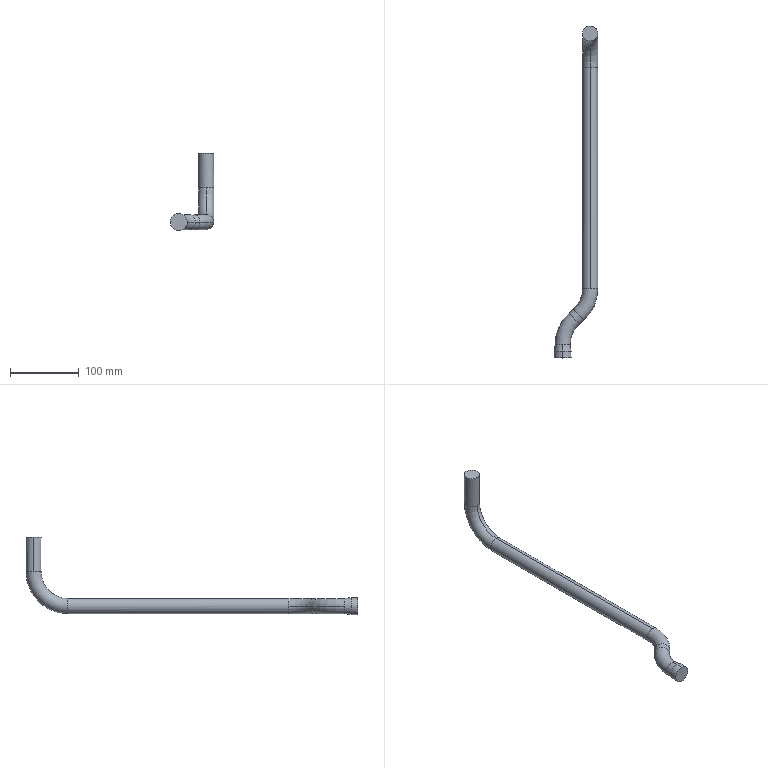Part | STEP file | copper tube 42_default_machined_ | 1 solid | 18 faces | box 63.3 x 483.405 x 112.3 mm | volume 215626 mm3 | cylinder 8 | torus 6 | cone 2 | plane 2 | commonest cylinder face diameters 22 x6 24.6 x2
STEP:
#1=CARTESIAN_POINT('',(0.,0.,0.));
#2=DIRECTION('',(0.,0.,1.));
#3=DIRECTION('',(1.,0.,0.));
#4=AXIS2_PLACEMENT_3D('',#1,#2,#3);
#5=CARTESIAN_POINT('',(380.2,1004.975,11.));
#6=VERTEX_POINT('',#5);
#7=CARTESIAN_POINT('',(380.2,1004.975,-11.));
#8=VERTEX_POINT('',#7);
#9=CARTESIAN_POINT('',(380.2,1004.975,0.));
#10=DIRECTION('',(0.,1.,0.));
#11=DIRECTION('',(-1.,0.,0.));
#12=AXIS2_PLACEMENT_3D('',#9,#10,#11);
#13=CIRCLE('',#12,11.);
#14=CARTESIAN_POINT('',(380.2,1004.975,50.));
#15=DIRECTION('',(1.,0.,0.));
#16=DIRECTION('',(0.,0.,-1.));
#17=AXIS2_PLACEMENT_3D('',#14,#15,#16);
#18=TOROIDAL_SURFACE('',#17,50.,11.);
#19=CARTESIAN_POINT('',(0.,4.712));
#20=DIRECTION('',(0.,-1.));
#21=VECTOR('',#20,1.);
#22=LINE('',#19,#21);
#23=(GEOMETRIC_REPRESENTATION_CONTEXT(2)PARAMETRIC_REPRESENTATION_CONTEXT()REPRESENTATION_CONTEXT('',''));
#24=DEFINITIONAL_REPRESENTATION('',(#22),#23);
#25=PCURVE('',#18,#24);
#26=CARTESIAN_POINT('',(380.2,683.041,0.));
#27=DIRECTION('',(0.,1.,0.));
#28=DIRECTION('',(0.,0.,1.));
#29=AXIS2_PLACEMENT_3D('',#26,#27,#28);
#30=CYLINDRICAL_SURFACE('',#29,11.);
#31=CARTESIAN_POINT('',(-1.571,321.934));
#32=DIRECTION('',(1.,0.));
#33=VECTOR('',#32,1.);
#34=LINE('',#31,#33);
#35=(GEOMETRIC_REPRESENTATION_CONTEXT(2)PARAMETRIC_REPRESENTATION_CONTEXT()REPRESENTATION_CONTEXT('',''));
#36=DEFINITIONAL_REPRESENTATION('',(#34),#35);
#37=PCURVE('',#30,#36);
#38=SURFACE_CURVE('',#13,(#25,#37),.PCURVE_S1.);
#39=EDGE_CURVE('',#6,#8,#38,.T.);
#40=ORIENTED_EDGE('',*,*,#39,.T.);
#41=CARTESIAN_POINT('',(380.2,1065.975,50.));
#42=VERTEX_POINT('',#41);
#43=CARTESIAN_POINT('',(380.2,1004.975,50.));
#44=DIRECTION('',(1.,0.,0.));
#45=DIRECTION('',(0.,0.,-1.));
#46=AXIS2_PLACEMENT_3D('',#43,#44,#45);
#47=CIRCLE('',#46,61.);
#48=CARTESIAN_POINT('',(0.,0.));
#49=DIRECTION('',(1.,0.));
#50=VECTOR('',#49,1.);
#51=LINE('',#48,#50);
#52=(GEOMETRIC_REPRESENTATION_CONTEXT(2)PARAMETRIC_REPRESENTATION_CONTEXT()REPRESENTATION_CONTEXT('',''));
#53=DEFINITIONAL_REPRESENTATION('',(#51),#52);
#54=PCURVE('',#18,#53);
#55=CARTESIAN_POINT('',(380.2,1004.975,50.));
#56=DIRECTION('',(1.,0.,0.));
#57=DIRECTION('',(0.,0.,-1.));
#58=AXIS2_PLACEMENT_3D('',#55,#56,#57);
#59=TOROIDAL_SURFACE('',#58,50.,11.);
#60=CARTESIAN_POINT('',(0.,6.283));
#61=DIRECTION('',(1.,0.));
#62=VECTOR('',#61,1.);
#63=LINE('',#60,#62);
#64=(GEOMETRIC_REPRESENTATION_CONTEXT(2)PARAMETRIC_REPRESENTATION_CONTEXT()REPRESENTATION_CONTEXT('',''));
#65=DEFINITIONAL_REPRESENTATION('',(#63),#64);
#66=PCURVE('',#59,#65);
#67=SURFACE_CURVE('',#47,(#54,#66),.PCURVE_S1.);
#68=EDGE_CURVE('',#8,#42,#67,.T.);
#69=ORIENTED_EDGE('',*,*,#68,.T.);
#70=CARTESIAN_POINT('',(391.2,1054.975,50.));
#71=VERTEX_POINT('',#70);
#72=CARTESIAN_POINT('',(380.2,1054.975,50.));
#73=DIRECTION('',(0.,0.,1.));
#74=DIRECTION('',(-1.,0.,0.));
#75=AXIS2_PLACEMENT_3D('',#72,#73,#74);
#76=CIRCLE('',#75,11.);
#77=CARTESIAN_POINT('',(1.571,4.712));
#78=DIRECTION('',(0.,-1.));
#79=VECTOR('',#78,1.);
#80=LINE('',#77,#79);
#81=(GEOMETRIC_REPRESENTATION_CONTEXT(2)PARAMETRIC_REPRESENTATION_CONTEXT()REPRESENTATION_CONTEXT('',''));
#82=DEFINITIONAL_REPRESENTATION('',(#80),#81);
#83=PCURVE('',#18,#82);
#84=CARTESIAN_POINT('',(380.2,1054.975,50.));
#85=DIRECTION('',(0.,0.,1.));
#86=DIRECTION('',(1.,0.,0.));
#87=AXIS2_PLACEMENT_3D('',#84,#85,#86);
#88=CYLINDRICAL_SURFACE('',#87,11.);
#89=CARTESIAN_POINT('',(-3.142,0.));
#90=DIRECTION('',(1.,0.));
#91=VECTOR('',#90,1.);
#92=LINE('',#89,#91);
#93=(GEOMETRIC_REPRESENTATION_CONTEXT(2)PARAMETRIC_REPRESENTATION_CONTEXT()REPRESENTATION_CONTEXT('',''));
#94=DEFINITIONAL_REPRESENTATION('',(#92),#93);
#95=PCURVE('',#88,#94);
#96=SURFACE_CURVE('',#76,(#83,#95),.PCURVE_S1.);
#97=EDGE_CURVE('',#71,#42,#96,.T.);
#98=ORIENTED_EDGE('',*,*,#97,.F.);
#99=CARTESIAN_POINT('',(380.2,1043.975,50.));
#100=VERTEX_POINT('',#99);
#101=CARTESIAN_POINT('',(380.2,1054.975,50.));
#102=DIRECTION('',(0.,0.,1.));
#103=DIRECTION('',(-1.,0.,0.));
#104=AXIS2_PLACEMENT_3D('',#101,#102,#103);
#105=CIRCLE('',#104,11.);
#106=CARTESIAN_POINT('',(1.571,4.712));
#107=DIRECTION('',(0.,-1.));
#108=VECTOR('',#107,1.);
#109=LINE('',#106,#108);
#110=(GEOMETRIC_REPRESENTATION_CONTEXT(2)PARAMETRIC_REPRESENTATION_CONTEXT()REPRESENTATION_CONTEXT('',''));
#111=DEFINITIONAL_REPRESENTATION('',(#109),#110);
#112=PCURVE('',#18,#111);
#113=CARTESIAN_POINT('',(380.2,1054.975,50.));
#114=DIRECTION('',(0.,0.,1.));
#115=DIRECTION('',(1.,0.,0.));
#116=AXIS2_PLACEMENT_3D('',#113,#114,#115);
#117=CYLINDRICAL_SURFACE('',#116,11.);
#118=CARTESIAN_POINT('',(3.142,0.));
#119=DIRECTION('',(1.,0.));
#120=VECTOR('',#119,1.);
#121=LINE('',#118,#120);
#122=(GEOMETRIC_REPRESENTATION_CONTEXT(2)PARAMETRIC_REPRESENTATION_CONTEXT()REPRESENTATION_CONTEXT('',''));
#123=DEFINITIONAL_REPRESENTATION('',(#121),#122);
#124=PCURVE('',#117,#123);
#125=SURFACE_CURVE('',#105,(#112,#124),.PCURVE_S1.);
#126=EDGE_CURVE('',#100,#71,#125,.T.);
#127=ORIENTED_EDGE('',*,*,#126,.F.);
#128=CARTESIAN_POINT('',(380.2,1004.975,50.));
#129=DIRECTION('',(1.,0.,0.));
#130=DIRECTION('',(0.,0.,-1.));
#131=AXIS2_PLACEMENT_3D('',#128,#129,#130);
#132=CIRCLE('',#131,39.);
#133=CARTESIAN_POINT('',(0.,3.142));
#134=DIRECTION('',(1.,0.));
#135=VECTOR('',#134,1.);
#136=LINE('',#133,#135);
#137=(GEOMETRIC_REPRESENTATION_CONTEXT(2)PARAMETRIC_REPRESENTATION_CONTEXT()REPRESENTATION_CONTEXT('',''));
#138=DEFINITIONAL_REPRESENTATION('',(#136),#137);
#139=PCURVE('',#18,#138);
#140=CARTESIAN_POINT('',(0.,3.142));
#141=DIRECTION('',(1.,0.));
#142=VECTOR('',#141,1.);
#143=LINE('',#140,#142);
#144=(GEOMETRIC_REPRESENTATION_CONTEXT(2)PARAMETRIC_REPRESENTATION_CONTEXT()REPRESENTATION_CONTEXT('',''));
#145=DEFINITIONAL_REPRESENTATION('',(#143),#144);
#146=PCURVE('',#59,#145);
#147=SURFACE_CURVE('',#132,(#139,#146),.PCURVE_S1.);
#148=EDGE_CURVE('',#6,#100,#147,.T.);
#149=ORIENTED_EDGE('',*,*,#148,.F.);
#150=EDGE_LOOP('',(#40,#69,#98,#127,#149));
#151=FACE_BOUND('',#150,.T.);
#152=ADVANCED_FACE('',(#151),#18,.T.);
#153=CARTESIAN_POINT('',(340.2,602.57,-11.));
#154=VERTEX_POINT('',#153);
#155=CARTESIAN_POINT('',(329.2,602.57,0.));
#156=VERTEX_POINT('',#155);
#157=CARTESIAN_POINT('',(340.2,602.57,0.));
#158=DIRECTION('',(0.,1.,0.));
#159=DIRECTION('',(0.,0.,-1.));
#160=AXIS2_PLACEMENT_3D('',#157,#158,#159);
#161=CIRCLE('',#160,11.);
#162=CARTESIAN_POINT('',(390.2,602.57,0.));
#163=DIRECTION('',(0.,0.,-1.));
#164=DIRECTION('',(-1.,0.,0.));
#165=AXIS2_PLACEMENT_3D('',#162,#163,#164);
#166=TOROIDAL_SURFACE('',#165,50.,11.);
#167=CARTESIAN_POINT('',(0.,1.571));
#168=DIRECTION('',(0.,-1.));
#169=VECTOR('',#168,1.);
#170=LINE('',#167,#169);
#171=(GEOMETRIC_REPRESENTATION_CONTEXT(2)PARAMETRIC_REPRESENTATION_CONTEXT()REPRESENTATION_CONTEXT('',''));
#172=DEFINITIONAL_REPRESENTATION('',(#170),#171);
#173=PCURVE('',#166,#172);
#174=CARTESIAN_POINT('',(340.2,592.57,0.));
#175=DIRECTION('',(0.,-1.,0.));
#176=DIRECTION('',(0.,0.,-1.));
#177=AXIS2_PLACEMENT_3D('',#174,#175,#176);
#178=CONICAL_SURFACE('',#177,12.3,0.1293);
#179=CARTESIAN_POINT('',(6.283,-10.));
#180=DIRECTION('',(-1.,0.));
#181=VECTOR('',#180,1.);
#182=LINE('',#179,#181);
#183=(GEOMETRIC_REPRESENTATION_CONTEXT(2)PARAMETRIC_REPRESENTATION_CONTEXT()REPRESENTATION_CONTEXT('',''));
#184=DEFINITIONAL_REPRESENTATION('',(#182),#183);
#185=PCURVE('',#178,#184);
#186=SURFACE_CURVE('',#161,(#173,#185),.PCURVE_S1.);
#187=EDGE_CURVE('',#154,#156,#186,.T.);
#188=ORIENTED_EDGE('',*,*,#187,.T.);
#189=CARTESIAN_POINT('',(349.639,648.131,0.));
#190=VERTEX_POINT('',#189);
#191=CARTESIAN_POINT('',(390.2,602.57,0.));
#192=DIRECTION('',(0.,0.,-1.));
#193=DIRECTION('',(-1.,0.,0.));
#194=AXIS2_PLACEMENT_3D('',#191,#192,#193);
#195=CIRCLE('',#194,61.);
#196=CARTESIAN_POINT('',(0.,0.));
#197=DIRECTION('',(1.,0.));
#198=VECTOR('',#197,1.);
#199=LINE('',#196,#198);
#200=(GEOMETRIC_REPRESENTATION_CONTEXT(2)PARAMETRIC_REPRESENTATION_CONTEXT()REPRESENTATION_CONTEXT('',''));
#201=DEFINITIONAL_REPRESENTATION('',(#199),#200);
#202=PCURVE('',#166,#201);
#203=CARTESIAN_POINT('',(390.2,602.57,0.));
#204=DIRECTION('',(0.,0.,-1.));
#205=DIRECTION('',(-1.,0.,0.));
#206=AXIS2_PLACEMENT_3D('',#203,#204,#205);
#207=TOROIDAL_SURFACE('',#206,50.,11.);
#208=CARTESIAN_POINT('',(0.,6.283));
#209=DIRECTION('',(1.,0.));
#210=VECTOR('',#209,1.);
#211=LINE('',#208,#210);
#212=(GEOMETRIC_REPRESENTATION_CONTEXT(2)PARAMETRIC_REPRESENTATION_CONTEXT()REPRESENTATION_CONTEXT('',''));
#213=DEFINITIONAL_REPRESENTATION('',(#211),#212);
#214=PCURVE('',#207,#213);
#215=SURFACE_CURVE('',#195,(#202,#214),.PCURVE_S1.);
#216=EDGE_CURVE('',#156,#190,#215,.T.);
#217=ORIENTED_EDGE('',*,*,#216,.T.);
#218=CARTESIAN_POINT('',(364.268,631.699,0.));
#219=VERTEX_POINT('',#218);
#220=CARTESIAN_POINT('',(356.953,639.915,0.));
#221=DIRECTION('',(0.7469,0.6649,0.));
#222=DIRECTION('',(-0.6649,0.7469,0.));
#223=AXIS2_PLACEMENT_3D('',#220,#221,#222);
#224=CIRCLE('',#223,11.);
#225=CARTESIAN_POINT('',(0.8434,6.283));
#226=DIRECTION('',(0.,-1.));
#227=VECTOR('',#226,1.);
#228=LINE('',#225,#227);
#229=(GEOMETRIC_REPRESENTATION_CONTEXT(2)PARAMETRIC_REPRESENTATION_CONTEXT()REPRESENTATION_CONTEXT('',''));
#230=DEFINITIONAL_REPRESENTATION('',(#228),#229);
#231=PCURVE('',#166,#230);
#232=CARTESIAN_POINT('',(356.953,639.915,0.));
#233=DIRECTION('',(0.7469,0.6649,0.));
#234=DIRECTION('',(-0.6649,0.7469,0.));
#235=AXIS2_PLACEMENT_3D('',#232,#233,#234);
#236=CYLINDRICAL_SURFACE('',#235,11.);
#237=CARTESIAN_POINT('',(0.,0.));
#238=DIRECTION('',(1.,0.));
#239=VECTOR('',#238,1.);
#240=LINE('',#237,#239);
#241=(GEOMETRIC_REPRESENTATION_CONTEXT(2)PARAMETRIC_REPRESENTATION_CONTEXT()REPRESENTATION_CONTEXT('',''));
#242=DEFINITIONAL_REPRESENTATION('',(#240),#241);
#243=PCURVE('',#236,#242);
#244=SURFACE_CURVE('',#224,(#231,#243),.PCURVE_S1.);
#245=EDGE_CURVE('',#219,#190,#244,.T.);
#246=ORIENTED_EDGE('',*,*,#245,.F.);
#247=CARTESIAN_POINT('',(351.2,602.57,0.));
#248=VERTEX_POINT('',#247);
#249=CARTESIAN_POINT('',(390.2,602.57,0.));
#250=DIRECTION('',(0.,0.,-1.));
#251=DIRECTION('',(-1.,0.,0.));
#252=AXIS2_PLACEMENT_3D('',#249,#250,#251);
#253=CIRCLE('',#252,39.);
#254=CARTESIAN_POINT('',(0.,3.142));
#255=DIRECTION('',(1.,0.));
#256=VECTOR('',#255,1.);
#257=LINE('',#254,#256);
#258=(GEOMETRIC_REPRESENTATION_CONTEXT(2)PARAMETRIC_REPRESENTATION_CONTEXT()REPRESENTATION_CONTEXT('',''));
#259=DEFINITIONAL_REPRESENTATION('',(#257),#258);
#260=PCURVE('',#166,#259);
#261=CARTESIAN_POINT('',(0.,3.142));
#262=DIRECTION('',(1.,0.));
#263=VECTOR('',#262,1.);
#264=LINE('',#261,#263);
#265=(GEOMETRIC_REPRESENTATION_CONTEXT(2)PARAMETRIC_REPRESENTATION_CONTEXT()REPRESENTATION_CONTEXT('',''));
#266=DEFINITIONAL_REPRESENTATION('',(#264),#265);
#267=PCURVE('',#207,#266);
#268=SURFACE_CURVE('',#253,(#260,#267),.PCURVE_S1.);
#269=EDGE_CURVE('',#248,#219,#268,.T.);
#270=ORIENTED_EDGE('',*,*,#269,.F.);
#271=CARTESIAN_POINT('',(340.2,602.57,0.));
#272=DIRECTION('',(0.,1.,0.));
#273=DIRECTION('',(0.,0.,-1.));
#274=AXIS2_PLACEMENT_3D('',#271,#272,#273);
#275=CIRCLE('',#274,11.);
#276=CARTESIAN_POINT('',(0.,7.854));
#277=DIRECTION('',(0.,-1.));
#278=VECTOR('',#277,1.);
#279=LINE('',#276,#278);
#280=(GEOMETRIC_REPRESENTATION_CONTEXT(2)PARAMETRIC_REPRESENTATION_CONTEXT()REPRESENTATION_CONTEXT('',''));
#281=DEFINITIONAL_REPRESENTATION('',(#279),#280);
#282=PCURVE('',#166,#281);
#283=CARTESIAN_POINT('',(340.2,592.57,0.));
#284=DIRECTION('',(0.,-1.,0.));
#285=DIRECTION('',(0.,0.,-1.));
#286=AXIS2_PLACEMENT_3D('',#283,#284,#285);
#287=CONICAL_SURFACE('',#286,12.3,0.1293);
#288=CARTESIAN_POINT('',(6.283,-10.));
#289=DIRECTION('',(-1.,0.));
#290=VECTOR('',#289,1.);
#291=LINE('',#288,#290);
#292=(GEOMETRIC_REPRESENTATION_CONTEXT(2)PARAMETRIC_REPRESENTATION_CONTEXT()REPRESENTATION_CONTEXT('',''));
#293=DEFINITIONAL_REPRESENTATION('',(#291),#292);
#294=PCURVE('',#287,#293);
#295=SURFACE_CURVE('',#275,(#282,#294),.PCURVE_S1.);
#296=EDGE_CURVE('',#248,#154,#295,.T.);
#297=ORIENTED_EDGE('',*,*,#296,.T.);
#298=EDGE_LOOP('',(#188,#217,#246,#270,#297));
#299=FACE_BOUND('',#298,.T.);
#300=ADVANCED_FACE('',(#299),#166,.T.);
#301=CARTESIAN_POINT('',(356.132,653.912,0.));
#302=VERTEX_POINT('',#301);
#303=CARTESIAN_POINT('',(370.761,637.48,0.));
#304=VERTEX_POINT('',#303);
#305=CARTESIAN_POINT('',(363.447,645.696,0.));
#306=DIRECTION('',(0.7469,0.6649,0.));
#307=DIRECTION('',(-0.6649,0.7469,0.));
#308=AXIS2_PLACEMENT_3D('',#305,#306,#307);
#309=CIRCLE('',#308,11.);
#310=CARTESIAN_POINT('',(330.2,683.041,0.));
#311=DIRECTION('',(0.,0.,1.));
#312=DIRECTION('',(1.,0.,0.));
#313=AXIS2_PLACEMENT_3D('',#310,#311,#312);
#314=TOROIDAL_SURFACE('',#313,50.,11.);
#315=CARTESIAN_POINT('',(5.44,3.142));
#316=DIRECTION('',(0.,-1.));
#317=VECTOR('',#316,1.);
#318=LINE('',#315,#317);
#319=(GEOMETRIC_REPRESENTATION_CONTEXT(2)PARAMETRIC_REPRESENTATION_CONTEXT()REPRESENTATION_CONTEXT('',''));
#320=DEFINITIONAL_REPRESENTATION('',(#318),#319);
#321=PCURVE('',#314,#320);
#322=CARTESIAN_POINT('',(356.953,639.915,0.));
#323=DIRECTION('',(0.7469,0.6649,0.));
#324=DIRECTION('',(-0.6649,0.7469,0.));
#325=AXIS2_PLACEMENT_3D('',#322,#323,#324);
#326=CYLINDRICAL_SURFACE('',#325,11.);
#327=CARTESIAN_POINT('',(0.,8.694));
#328=DIRECTION('',(1.,0.));
#329=VECTOR('',#328,1.);
#330=LINE('',#327,#329);
#331=(GEOMETRIC_REPRESENTATION_CONTEXT(2)PARAMETRIC_REPRESENTATION_CONTEXT()REPRESENTATION_CONTEXT('',''));
#332=DEFINITIONAL_REPRESENTATION('',(#330),#331);
#333=PCURVE('',#326,#332);
#334=SURFACE_CURVE('',#309,(#321,#333),.PCURVE_S1.);
#335=EDGE_CURVE('',#302,#304,#334,.T.);
#336=ORIENTED_EDGE('',*,*,#335,.T.);
#337=CARTESIAN_POINT('',(391.2,683.041,0.));
#338=VERTEX_POINT('',#337);
#339=CARTESIAN_POINT('',(330.2,683.041,0.));
#340=DIRECTION('',(0.,0.,1.));
#341=DIRECTION('',(1.,0.,0.));
#342=AXIS2_PLACEMENT_3D('',#339,#340,#341);
#343=CIRCLE('',#342,61.);
#344=CARTESIAN_POINT('',(0.,0.));
#345=DIRECTION('',(1.,0.));
#346=VECTOR('',#345,1.);
#347=LINE('',#344,#346);
#348=(GEOMETRIC_REPRESENTATION_CONTEXT(2)PARAMETRIC_REPRESENTATION_CONTEXT()REPRESENTATION_CONTEXT('',''));
#349=DEFINITIONAL_REPRESENTATION('',(#347),#348);
#350=PCURVE('',#314,#349);
#351=CARTESIAN_POINT('',(330.2,683.041,0.));
#352=DIRECTION('',(0.,0.,1.));
#353=DIRECTION('',(1.,0.,0.));
#354=AXIS2_PLACEMENT_3D('',#351,#352,#353);
#355=TOROIDAL_SURFACE('',#354,50.,11.);
#356=CARTESIAN_POINT('',(0.,6.283));
#357=DIRECTION('',(1.,0.));
#358=VECTOR('',#357,1.);
#359=LINE('',#356,#358);
#360=(GEOMETRIC_REPRESENTATION_CONTEXT(2)PARAMETRIC_REPRESENTATION_CONTEXT()REPRESENTATION_CONTEXT('',''));
#361=DEFINITIONAL_REPRESENTATION('',(#359),#360);
#362=PCURVE('',#355,#361);
#363=SURFACE_CURVE('',#343,(#350,#362),.PCURVE_S1.);
#364=EDGE_CURVE('',#304,#338,#363,.T.);
#365=ORIENTED_EDGE('',*,*,#364,.T.);
#366=CARTESIAN_POINT('',(380.2,683.041,11.));
#367=VERTEX_POINT('',#366);
#368=CARTESIAN_POINT('',(380.2,683.041,0.));
#369=DIRECTION('',(0.,1.,0.));
#370=DIRECTION('',(-1.,0.,0.));
#371=AXIS2_PLACEMENT_3D('',#368,#369,#370);
#372=CIRCLE('',#371,11.);
#373=CARTESIAN_POINT('',(6.283,3.142));
#374=DIRECTION('',(0.,-1.));
#375=VECTOR('',#374,1.);
#376=LINE('',#373,#375);
#377=(GEOMETRIC_REPRESENTATION_CONTEXT(2)PARAMETRIC_REPRESENTATION_CONTEXT()REPRESENTATION_CONTEXT('',''));
#378=DEFINITIONAL_REPRESENTATION('',(#376),#377);
#379=PCURVE('',#314,#378);
#380=CARTESIAN_POINT('',(-1.571,0.));
#381=DIRECTION('',(1.,0.));
#382=VECTOR('',#381,1.);
#383=LINE('',#380,#382);
#384=(GEOMETRIC_REPRESENTATION_CONTEXT(2)PARAMETRIC_REPRESENTATION_CONTEXT()REPRESENTATION_CONTEXT('',''));
#385=DEFINITIONAL_REPRESENTATION('',(#383),#384);
#386=PCURVE('',#30,#385);
#387=SURFACE_CURVE('',#372,(#379,#386),.PCURVE_S1.);
#388=EDGE_CURVE('',#367,#338,#387,.T.);
#389=ORIENTED_EDGE('',*,*,#388,.F.);
#390=CARTESIAN_POINT('',(369.2,683.041,0.));
#391=VERTEX_POINT('',#390);
#392=CARTESIAN_POINT('',(380.2,683.041,0.));
#393=DIRECTION('',(0.,1.,0.));
#394=DIRECTION('',(-1.,0.,0.));
#395=AXIS2_PLACEMENT_3D('',#392,#393,#394);
#396=CIRCLE('',#395,11.);
#397=CARTESIAN_POINT('',(6.283,3.142));
#398=DIRECTION('',(0.,-1.));
#399=VECTOR('',#398,1.);
#400=LINE('',#397,#399);
#401=(GEOMETRIC_REPRESENTATION_CONTEXT(2)PARAMETRIC_REPRESENTATION_CONTEXT()REPRESENTATION_CONTEXT('',''));
#402=DEFINITIONAL_REPRESENTATION('',(#400),#401);
#403=PCURVE('',#314,#402);
#404=CARTESIAN_POINT('',(380.2,683.041,0.));
#405=DIRECTION('',(0.,1.,0.));
#406=DIRECTION('',(0.,0.,1.));
#407=AXIS2_PLACEMENT_3D('',#404,#405,#406);
#408=CYLINDRICAL_SURFACE('',#407,11.);
#409=CARTESIAN_POINT('',(4.712,0.));
#410=DIRECTION('',(1.,0.));
#411=VECTOR('',#410,1.);
#412=LINE('',#409,#411);
#413=(GEOMETRIC_REPRESENTATION_CONTEXT(2)PARAMETRIC_REPRESENTATION_CONTEXT()REPRESENTATION_CONTEXT('',''));
#414=DEFINITIONAL_REPRESENTATION('',(#412),#413);
#415=PCURVE('',#408,#414);
#416=SURFACE_CURVE('',#396,(#403,#415),.PCURVE_S1.);
#417=EDGE_CURVE('',#391,#367,#416,.T.);
#418=ORIENTED_EDGE('',*,*,#417,.F.);
#419=CARTESIAN_POINT('',(330.2,683.041,0.));
#420=DIRECTION('',(0.,0.,1.));
#421=DIRECTION('',(1.,0.,0.));
#422=AXIS2_PLACEMENT_3D('',#419,#420,#421);
#423=CIRCLE('',#422,39.);
#424=CARTESIAN_POINT('',(0.,3.142));
#425=DIRECTION('',(1.,0.));
#426=VECTOR('',#425,1.);
#427=LINE('',#424,#426);
#428=(GEOMETRIC_REPRESENTATION_CONTEXT(2)PARAMETRIC_REPRESENTATION_CONTEXT()REPRESENTATION_CONTEXT('',''));
#429=DEFINITIONAL_REPRESENTATION('',(#427),#428);
#430=PCURVE('',#314,#429);
#431=CARTESIAN_POINT('',(0.,3.142));
#432=DIRECTION('',(1.,0.));
#433=VECTOR('',#432,1.);
#434=LINE('',#431,#433);
#435=(GEOMETRIC_REPRESENTATION_CONTEXT(2)PARAMETRIC_REPRESENTATION_CONTEXT()REPRESENTATION_CONTEXT('',''));
#436=DEFINITIONAL_REPRESENTATION('',(#434),#435);
#437=PCURVE('',#355,#436);
#438=SURFACE_CURVE('',#423,(#430,#437),.PCURVE_S1.);
#439=EDGE_CURVE('',#302,#391,#438,.T.);
#440=ORIENTED_EDGE('',*,*,#439,.F.);
#441=EDGE_LOOP('',(#336,#365,#389,#418,#440));
#442=FACE_BOUND('',#441,.T.);
#443=ADVANCED_FACE('',(#442),#314,.T.);
#444=CARTESIAN_POINT('',(340.2,602.57,11.));
#445=VERTEX_POINT('',#444);
#446=CARTESIAN_POINT('',(340.2,602.57,0.));
#447=DIRECTION('',(0.,1.,0.));
#448=DIRECTION('',(0.,0.,-1.));
#449=AXIS2_PLACEMENT_3D('',#446,#447,#448);
#450=CIRCLE('',#449,11.);
#451=CARTESIAN_POINT('',(6.283,-10.));
#452=DIRECTION('',(-1.,0.));
#453=VECTOR('',#452,1.);
#454=LINE('',#451,#453);
#455=(GEOMETRIC_REPRESENTATION_CONTEXT(2)PARAMETRIC_REPRESENTATION_CONTEXT()REPRESENTATION_CONTEXT('',''));
#456=DEFINITIONAL_REPRESENTATION('',(#454),#455);
#457=PCURVE('',#287,#456);
#458=CARTESIAN_POINT('',(0.,7.854));
#459=DIRECTION('',(0.,-1.));
#460=VECTOR('',#459,1.);
#461=LINE('',#458,#460);
#462=(GEOMETRIC_REPRESENTATION_CONTEXT(2)PARAMETRIC_REPRESENTATION_CONTEXT()REPRESENTATION_CONTEXT('',''));
#463=DEFINITIONAL_REPRESENTATION('',(#461),#462);
#464=PCURVE('',#207,#463);
#465=SURFACE_CURVE('',#450,(#457,#464),.PCURVE_S1.);
#466=EDGE_CURVE('',#445,#248,#465,.T.);
#467=ORIENTED_EDGE('',*,*,#466,.F.);
#468=CARTESIAN_POINT('',(340.2,592.57,12.3));
#469=VERTEX_POINT('',#468);
#470=CARTESIAN_POINT('',(340.2,592.57,12.3));
#471=DIRECTION('',(0.,-0.9917,0.1289));
#472=VECTOR('',#471,1.);
#473=LINE('',#470,#472);
#474=CARTESIAN_POINT('',(3.142,0.));
#475=DIRECTION('',(0.,1.));
#476=VECTOR('',#475,1.);
#477=LINE('',#474,#476);
#478=(GEOMETRIC_REPRESENTATION_CONTEXT(2)PARAMETRIC_REPRESENTATION_CONTEXT()REPRESENTATION_CONTEXT('',''));
#479=DEFINITIONAL_REPRESENTATION('',(#477),#478);
#480=PCURVE('',#287,#479);
#481=CARTESIAN_POINT('',(3.142,0.));
#482=DIRECTION('',(0.,1.));
#483=VECTOR('',#482,1.);
#484=LINE('',#481,#483);
#485=(GEOMETRIC_REPRESENTATION_CONTEXT(2)PARAMETRIC_REPRESENTATION_CONTEXT()REPRESENTATION_CONTEXT('',''));
#486=DEFINITIONAL_REPRESENTATION('',(#484),#485);
#487=PCURVE('',#178,#486);
#488=SURFACE_CURVE('',#473,(#480,#487),.PCURVE_S1.);
#489=EDGE_CURVE('',#445,#469,#488,.T.);
#490=ORIENTED_EDGE('',*,*,#489,.T.);
#491=CARTESIAN_POINT('',(340.2,592.57,-12.3));
#492=VERTEX_POINT('',#491);
#493=CARTESIAN_POINT('',(340.2,592.57,0.));
#494=DIRECTION('',(0.,-1.,0.));
#495=DIRECTION('',(0.,0.,-1.));
#496=AXIS2_PLACEMENT_3D('',#493,#494,#495);
#497=CIRCLE('',#496,12.3);
#498=CARTESIAN_POINT('',(0.,0.));
#499=DIRECTION('',(1.,0.));
#500=VECTOR('',#499,1.);
#501=LINE('',#498,#500);
#502=(GEOMETRIC_REPRESENTATION_CONTEXT(2)PARAMETRIC_REPRESENTATION_CONTEXT()REPRESENTATION_CONTEXT('',''));
#503=DEFINITIONAL_REPRESENTATION('',(#501),#502);
#504=PCURVE('',#287,#503);
#505=CARTESIAN_POINT('',(340.2,582.57,0.));
#506=DIRECTION('',(0.,1.,0.));
#507=DIRECTION('',(0.,0.,1.));
#508=AXIS2_PLACEMENT_3D('',#505,#506,#507);
#509=CYLINDRICAL_SURFACE('',#508,12.3);
#510=CARTESIAN_POINT('',(3.142,10.));
#511=DIRECTION('',(-1.,0.));
#512=VECTOR('',#511,1.);
#513=LINE('',#510,#512);
#514=(GEOMETRIC_REPRESENTATION_CONTEXT(2)PARAMETRIC_REPRESENTATION_CONTEXT()REPRESENTATION_CONTEXT('',''));
#515=DEFINITIONAL_REPRESENTATION('',(#513),#514);
#516=PCURVE('',#509,#515);
#517=SURFACE_CURVE('',#497,(#504,#516),.PCURVE_S1.);
#518=EDGE_CURVE('',#492,#469,#517,.T.);
#519=ORIENTED_EDGE('',*,*,#518,.F.);
#520=CARTESIAN_POINT('',(340.2,592.57,-12.3));
#521=DIRECTION('',(0.,-0.9917,-0.1289));
#522=VECTOR('',#521,1.);
#523=LINE('',#520,#522);
#524=CARTESIAN_POINT('',(0.,0.));
#525=DIRECTION('',(0.,1.));
#526=VECTOR('',#525,1.);
#527=LINE('',#524,#526);
#528=(GEOMETRIC_REPRESENTATION_CONTEXT(2)PARAMETRIC_REPRESENTATION_CONTEXT()REPRESENTATION_CONTEXT('',''));
#529=DEFINITIONAL_REPRESENTATION('',(#527),#528);
#530=PCURVE('',#287,#529);
#531=CARTESIAN_POINT('',(6.283,0.));
#532=DIRECTION('',(0.,1.));
#533=VECTOR('',#532,1.);
#534=LINE('',#531,#533);
#535=(GEOMETRIC_REPRESENTATION_CONTEXT(2)PARAMETRIC_REPRESENTATION_CONTEXT()REPRESENTATION_CONTEXT('',''));
#536=DEFINITIONAL_REPRESENTATION('',(#534),#535);
#537=PCURVE('',#178,#536);
#538=SURFACE_CURVE('',#523,(#530,#537),.PCURVE_S1.);
#539=EDGE_CURVE('',#154,#492,#538,.T.);
#540=ORIENTED_EDGE('',*,*,#539,.F.);
#541=ORIENTED_EDGE('',*,*,#296,.F.);
#542=EDGE_LOOP('',(#467,#490,#519,#540,#541));
#543=FACE_BOUND('',#542,.T.);
#544=ADVANCED_FACE('',(#543),#287,.T.);
#545=CARTESIAN_POINT('',(340.2,582.57,-12.3));
#546=VERTEX_POINT('',#545);
#547=CARTESIAN_POINT('',(340.2,582.57,12.3));
#548=VERTEX_POINT('',#547);
#549=CARTESIAN_POINT('',(340.2,582.57,0.));
#550=DIRECTION('',(0.,-1.,0.));
#551=DIRECTION('',(0.,0.,-1.));
#552=AXIS2_PLACEMENT_3D('',#549,#550,#551);
#553=CIRCLE('',#552,12.3);
#554=CARTESIAN_POINT('',(3.142,0.));
#555=DIRECTION('',(-1.,0.));
#556=VECTOR('',#555,1.);
#557=LINE('',#554,#556);
#558=(GEOMETRIC_REPRESENTATION_CONTEXT(2)PARAMETRIC_REPRESENTATION_CONTEXT()REPRESENTATION_CONTEXT('',''));
#559=DEFINITIONAL_REPRESENTATION('',(#557),#558);
#560=PCURVE('',#509,#559);
#561=CARTESIAN_POINT('',(340.2,582.57,0.));
#562=DIRECTION('',(0.,-1.,0.));
#563=DIRECTION('',(0.,0.,-1.));
#564=AXIS2_PLACEMENT_3D('',#561,#562,#563);
#565=PLANE('',#564);
#566=CARTESIAN_POINT('',(0.,0.));
#567=DIRECTION('',(1.,0.));
#568=AXIS2_PLACEMENT_2D('',#566,#567);
#569=CIRCLE('',#568,12.3);
#570=(GEOMETRIC_REPRESENTATION_CONTEXT(2)PARAMETRIC_REPRESENTATION_CONTEXT()REPRESENTATION_CONTEXT('',''));
#571=DEFINITIONAL_REPRESENTATION('',(#569),#570);
#572=PCURVE('',#565,#571);
#573=SURFACE_CURVE('',#553,(#560,#572),.PCURVE_S1.);
#574=EDGE_CURVE('',#546,#548,#573,.T.);
#575=ORIENTED_EDGE('',*,*,#574,.F.);
#576=CARTESIAN_POINT('',(340.2,582.57,-12.3));
#577=DIRECTION('',(0.,1.,0.));
#578=VECTOR('',#577,1.);
#579=LINE('',#576,#578);
#580=CARTESIAN_POINT('',(3.142,0.));
#581=DIRECTION('',(0.,1.));
#582=VECTOR('',#581,1.);
#583=LINE('',#580,#582);
#584=(GEOMETRIC_REPRESENTATION_CONTEXT(2)PARAMETRIC_REPRESENTATION_CONTEXT()REPRESENTATION_CONTEXT('',''));
#585=DEFINITIONAL_REPRESENTATION('',(#583),#584);
#586=PCURVE('',#509,#585);
#587=CARTESIAN_POINT('',(340.2,582.57,0.));
#588=DIRECTION('',(0.,1.,0.));
#589=DIRECTION('',(0.,0.,1.));
#590=AXIS2_PLACEMENT_3D('',#587,#588,#589);
#591=CYLINDRICAL_SURFACE('',#590,12.3);
#592=CARTESIAN_POINT('',(3.142,0.));
#593=DIRECTION('',(0.,1.));
#594=VECTOR('',#593,1.);
#595=LINE('',#592,#594);
#596=(GEOMETRIC_REPRESENTATION_CONTEXT(2)PARAMETRIC_REPRESENTATION_CONTEXT()REPRESENTATION_CONTEXT('',''));
#597=DEFINITIONAL_REPRESENTATION('',(#595),#596);
#598=PCURVE('',#591,#597);
#599=SURFACE_CURVE('',#579,(#586,#598),.PCURVE_S1.);
#600=EDGE_CURVE('',#546,#492,#599,.T.);
#601=ORIENTED_EDGE('',*,*,#600,.T.);
#602=ORIENTED_EDGE('',*,*,#518,.T.);
#603=CARTESIAN_POINT('',(340.2,582.57,12.3));
#604=DIRECTION('',(0.,1.,0.));
#605=VECTOR('',#604,1.);
#606=LINE('',#603,#605);
#607=CARTESIAN_POINT('',(0.,0.));
#608=DIRECTION('',(0.,1.));
#609=VECTOR('',#608,1.);
#610=LINE('',#607,#609);
#611=(GEOMETRIC_REPRESENTATION_CONTEXT(2)PARAMETRIC_REPRESENTATION_CONTEXT()REPRESENTATION_CONTEXT('',''));
#612=DEFINITIONAL_REPRESENTATION('',(#610),#611);
#613=PCURVE('',#509,#612);
#614=CARTESIAN_POINT('',(6.283,0.));
#615=DIRECTION('',(0.,1.));
#616=VECTOR('',#615,1.);
#617=LINE('',#614,#616);
#618=(GEOMETRIC_REPRESENTATION_CONTEXT(2)PARAMETRIC_REPRESENTATION_CONTEXT()REPRESENTATION_CONTEXT('',''));
#619=DEFINITIONAL_REPRESENTATION('',(#617),#618);
#620=PCURVE('',#591,#619);
#621=SURFACE_CURVE('',#606,(#613,#620),.PCURVE_S1.);
#622=EDGE_CURVE('',#548,#469,#621,.T.);
#623=ORIENTED_EDGE('',*,*,#622,.F.);
#624=EDGE_LOOP('',(#575,#601,#602,#623));
#625=FACE_BOUND('',#624,.T.);
#626=ADVANCED_FACE('',(#625),#509,.T.);
#627=ORIENTED_EDGE('',*,*,#97,.T.);
#628=CARTESIAN_POINT('',(369.2,1054.975,50.));
#629=VERTEX_POINT('',#628);
#630=CARTESIAN_POINT('',(380.2,1054.975,50.));
#631=DIRECTION('',(0.,0.,1.));
#632=DIRECTION('',(-1.,0.,0.));
#633=AXIS2_PLACEMENT_3D('',#630,#631,#632);
#634=CIRCLE('',#633,11.);
#635=CARTESIAN_POINT('',(-3.142,0.));
#636=DIRECTION('',(1.,0.));
#637=VECTOR('',#636,1.);
#638=LINE('',#635,#637);
#639=(GEOMETRIC_REPRESENTATION_CONTEXT(2)PARAMETRIC_REPRESENTATION_CONTEXT()REPRESENTATION_CONTEXT('',''));
#640=DEFINITIONAL_REPRESENTATION('',(#638),#639);
#641=PCURVE('',#88,#640);
#642=CARTESIAN_POINT('',(1.571,10.996));
#643=DIRECTION('',(0.,-1.));
#644=VECTOR('',#643,1.);
#645=LINE('',#642,#644);
#646=(GEOMETRIC_REPRESENTATION_CONTEXT(2)PARAMETRIC_REPRESENTATION_CONTEXT()REPRESENTATION_CONTEXT('',''));
#647=DEFINITIONAL_REPRESENTATION('',(#645),#646);
#648=PCURVE('',#59,#647);
#649=SURFACE_CURVE('',#634,(#641,#648),.PCURVE_S1.);
#650=EDGE_CURVE('',#42,#629,#649,.T.);
#651=ORIENTED_EDGE('',*,*,#650,.T.);
#652=CARTESIAN_POINT('',(369.2,1054.975,100.));
#653=VERTEX_POINT('',#652);
#654=CARTESIAN_POINT('',(369.2,1054.975,50.));
#655=DIRECTION('',(0.,0.,1.));
#656=VECTOR('',#655,1.);
#657=LINE('',#654,#656);
#658=CARTESIAN_POINT('',(3.142,0.));
#659=DIRECTION('',(0.,1.));
#660=VECTOR('',#659,1.);
#661=LINE('',#658,#660);
#662=(GEOMETRIC_REPRESENTATION_CONTEXT(2)PARAMETRIC_REPRESENTATION_CONTEXT()REPRESENTATION_CONTEXT('',''));
#663=DEFINITIONAL_REPRESENTATION('',(#661),#662);
#664=PCURVE('',#88,#663);
#665=CARTESIAN_POINT('',(3.142,0.));
#666=DIRECTION('',(0.,1.));
#667=VECTOR('',#666,1.);
#668=LINE('',#665,#667);
#669=(GEOMETRIC_REPRESENTATION_CONTEXT(2)PARAMETRIC_REPRESENTATION_CONTEXT()REPRESENTATION_CONTEXT('',''));
#670=DEFINITIONAL_REPRESENTATION('',(#668),#669);
#671=PCURVE('',#117,#670);
#672=SURFACE_CURVE('',#657,(#664,#671),.PCURVE_S1.);
#673=EDGE_CURVE('',#629,#653,#672,.T.);
#674=ORIENTED_EDGE('',*,*,#673,.T.);
#675=CARTESIAN_POINT('',(391.2,1054.975,100.));
#676=VERTEX_POINT('',#675);
#677=CARTESIAN_POINT('',(380.2,1054.975,100.));
#678=DIRECTION('',(0.,0.,1.));
#679=DIRECTION('',(-1.,0.,0.));
#680=AXIS2_PLACEMENT_3D('',#677,#678,#679);
#681=CIRCLE('',#680,11.);
#682=CARTESIAN_POINT('',(-3.142,50.));
#683=DIRECTION('',(1.,0.));
#684=VECTOR('',#683,1.);
#685=LINE('',#682,#684);
#686=(GEOMETRIC_REPRESENTATION_CONTEXT(2)PARAMETRIC_REPRESENTATION_CONTEXT()REPRESENTATION_CONTEXT('',''));
#687=DEFINITIONAL_REPRESENTATION('',(#685),#686);
#688=PCURVE('',#88,#687);
#689=CARTESIAN_POINT('',(380.2,1054.975,100.));
#690=DIRECTION('',(0.,0.,1.));
#691=DIRECTION('',(-1.,0.,0.));
#692=AXIS2_PLACEMENT_3D('',#689,#690,#691);
#693=PLANE('',#692);
#694=CARTESIAN_POINT('',(0.,0.));
#695=DIRECTION('',(1.,0.));
#696=AXIS2_PLACEMENT_2D('',#694,#695);
#697=CIRCLE('',#696,11.);
#698=(GEOMETRIC_REPRESENTATION_CONTEXT(2)PARAMETRIC_REPRESENTATION_CONTEXT()REPRESENTATION_CONTEXT('',''));
#699=DEFINITIONAL_REPRESENTATION('',(#697),#698);
#700=PCURVE('',#693,#699);
#701=SURFACE_CURVE('',#681,(#688,#700),.PCURVE_S1.);
#702=EDGE_CURVE('',#676,#653,#701,.T.);
#703=ORIENTED_EDGE('',*,*,#702,.F.);
#704=CARTESIAN_POINT('',(391.2,1054.975,50.));
#705=DIRECTION('',(0.,0.,1.));
#706=VECTOR('',#705,1.);
#707=LINE('',#704,#706);
#708=CARTESIAN_POINT('',(0.,0.));
#709=DIRECTION('',(0.,1.));
#710=VECTOR('',#709,1.);
#711=LINE('',#708,#710);
#712=(GEOMETRIC_REPRESENTATION_CONTEXT(2)PARAMETRIC_REPRESENTATION_CONTEXT()REPRESENTATION_CONTEXT('',''));
#713=DEFINITIONAL_REPRESENTATION('',(#711),#712);
#714=PCURVE('',#88,#713);
#715=CARTESIAN_POINT('',(6.283,0.));
#716=DIRECTION('',(0.,1.));
#717=VECTOR('',#716,1.);
#718=LINE('',#715,#717);
#719=(GEOMETRIC_REPRESENTATION_CONTEXT(2)PARAMETRIC_REPRESENTATION_CONTEXT()REPRESENTATION_CONTEXT('',''));
#720=DEFINITIONAL_REPRESENTATION('',(#718),#719);
#721=PCURVE('',#117,#720);
#722=SURFACE_CURVE('',#707,(#714,#721),.PCURVE_S1.);
#723=EDGE_CURVE('',#71,#676,#722,.T.);
#724=ORIENTED_EDGE('',*,*,#723,.F.);
#725=EDGE_LOOP('',(#627,#651,#674,#703,#724));
#726=FACE_BOUND('',#725,.T.);
#727=ADVANCED_FACE('',(#726),#88,.T.);
#728=CARTESIAN_POINT('',(356.953,639.915,0.));
#729=DIRECTION('',(0.7469,0.6649,0.));
#730=DIRECTION('',(-0.6649,0.7469,0.));
#731=AXIS2_PLACEMENT_3D('',#728,#729,#730);
#732=CIRCLE('',#731,11.);
#733=CARTESIAN_POINT('',(0.,0.));
#734=DIRECTION('',(1.,0.));
#735=VECTOR('',#734,1.);
#736=LINE('',#733,#735);
#737=(GEOMETRIC_REPRESENTATION_CONTEXT(2)PARAMETRIC_REPRESENTATION_CONTEXT()REPRESENTATION_CONTEXT('',''));
#738=DEFINITIONAL_REPRESENTATION('',(#736),#737);
#739=PCURVE('',#326,#738);
#740=CARTESIAN_POINT('',(0.8434,6.283));
#741=DIRECTION('',(0.,-1.));
#742=VECTOR('',#741,1.);
#743=LINE('',#740,#742);
#744=(GEOMETRIC_REPRESENTATION_CONTEXT(2)PARAMETRIC_REPRESENTATION_CONTEXT()REPRESENTATION_CONTEXT('',''));
#745=DEFINITIONAL_REPRESENTATION('',(#743),#744);
#746=PCURVE('',#207,#745);
#747=SURFACE_CURVE('',#732,(#739,#746),.PCURVE_S1.);
#748=EDGE_CURVE('',#190,#219,#747,.T.);
#749=ORIENTED_EDGE('',*,*,#748,.T.);
#750=CARTESIAN_POINT('',(364.268,631.699,0.));
#751=DIRECTION('',(0.7469,0.6649,0.));
#752=VECTOR('',#751,1.);
#753=LINE('',#750,#752);
#754=CARTESIAN_POINT('',(3.142,0.));
#755=DIRECTION('',(0.,1.));
#756=VECTOR('',#755,1.);
#757=LINE('',#754,#756);
#758=(GEOMETRIC_REPRESENTATION_CONTEXT(2)PARAMETRIC_REPRESENTATION_CONTEXT()REPRESENTATION_CONTEXT('',''));
#759=DEFINITIONAL_REPRESENTATION('',(#757),#758);
#760=PCURVE('',#326,#759);
#761=CARTESIAN_POINT('',(3.142,0.));
#762=DIRECTION('',(0.,1.));
#763=VECTOR('',#762,1.);
#764=LINE('',#761,#763);
#765=(GEOMETRIC_REPRESENTATION_CONTEXT(2)PARAMETRIC_REPRESENTATION_CONTEXT()REPRESENTATION_CONTEXT('',''));
#766=DEFINITIONAL_REPRESENTATION('',(#764),#765);
#767=PCURVE('',#236,#766);
#768=SURFACE_CURVE('',#753,(#760,#767),.PCURVE_S1.);
#769=EDGE_CURVE('',#219,#304,#768,.T.);
#770=ORIENTED_EDGE('',*,*,#769,.T.);
#771=ORIENTED_EDGE('',*,*,#335,.F.);
#772=CARTESIAN_POINT('',(349.639,648.131,0.));
#773=DIRECTION('',(0.7469,0.6649,0.));
#774=VECTOR('',#773,1.);
#775=LINE('',#772,#774);
#776=CARTESIAN_POINT('',(0.,0.));
#777=DIRECTION('',(0.,1.));
#778=VECTOR('',#777,1.);
#779=LINE('',#776,#778);
#780=(GEOMETRIC_REPRESENTATION_CONTEXT(2)PARAMETRIC_REPRESENTATION_CONTEXT()REPRESENTATION_CONTEXT('',''));
#781=DEFINITIONAL_REPRESENTATION('',(#779),#780);
#782=PCURVE('',#326,#781);
#783=CARTESIAN_POINT('',(6.283,0.));
#784=DIRECTION('',(0.,1.));
#785=VECTOR('',#784,1.);
#786=LINE('',#783,#785);
#787=(GEOMETRIC_REPRESENTATION_CONTEXT(2)PARAMETRIC_REPRESENTATION_CONTEXT()REPRESENTATION_CONTEXT('',''));
#788=DEFINITIONAL_REPRESENTATION('',(#786),#787);
#789=PCURVE('',#236,#788);
#790=SURFACE_CURVE('',#775,(#782,#789),.PCURVE_S1.);
#791=EDGE_CURVE('',#190,#302,#790,.T.);
#792=ORIENTED_EDGE('',*,*,#791,.F.);
#793=EDGE_LOOP('',(#749,#770,#771,#792));
#794=FACE_BOUND('',#793,.T.);
#795=ADVANCED_FACE('',(#794),#326,.T.);
#796=ORIENTED_EDGE('',*,*,#388,.T.);
#797=CARTESIAN_POINT('',(380.2,683.041,-11.));
#798=VERTEX_POINT('',#797);
#799=CARTESIAN_POINT('',(380.2,683.041,0.));
#800=DIRECTION('',(0.,1.,0.));
#801=DIRECTION('',(-1.,0.,0.));
#802=AXIS2_PLACEMENT_3D('',#799,#800,#801);
#803=CIRCLE('',#802,11.);
#804=CARTESIAN_POINT('',(-1.571,0.));
#805=DIRECTION('',(1.,0.));
#806=VECTOR('',#805,1.);
#807=LINE('',#804,#806);
#808=(GEOMETRIC_REPRESENTATION_CONTEXT(2)PARAMETRIC_REPRESENTATION_CONTEXT()REPRESENTATION_CONTEXT('',''));
#809=DEFINITIONAL_REPRESENTATION('',(#807),#808);
#810=PCURVE('',#30,#809);
#811=CARTESIAN_POINT('',(6.283,9.425));
#812=DIRECTION('',(0.,-1.));
#813=VECTOR('',#812,1.);
#814=LINE('',#811,#813);
#815=(GEOMETRIC_REPRESENTATION_CONTEXT(2)PARAMETRIC_REPRESENTATION_CONTEXT()REPRESENTATION_CONTEXT('',''));
#816=DEFINITIONAL_REPRESENTATION('',(#814),#815);
#817=PCURVE('',#355,#816);
#818=SURFACE_CURVE('',#803,(#810,#817),.PCURVE_S1.);
#819=EDGE_CURVE('',#338,#798,#818,.T.);
#820=ORIENTED_EDGE('',*,*,#819,.T.);
#821=CARTESIAN_POINT('',(380.2,683.041,-11.));
#822=DIRECTION('',(0.,1.,0.));
#823=VECTOR('',#822,1.);
#824=LINE('',#821,#823);
#825=CARTESIAN_POINT('',(3.142,0.));
#826=DIRECTION('',(0.,1.));
#827=VECTOR('',#826,1.);
#828=LINE('',#825,#827);
#829=(GEOMETRIC_REPRESENTATION_CONTEXT(2)PARAMETRIC_REPRESENTATION_CONTEXT()REPRESENTATION_CONTEXT('',''));
#830=DEFINITIONAL_REPRESENTATION('',(#828),#829);
#831=PCURVE('',#30,#830);
#832=CARTESIAN_POINT('',(3.142,0.));
#833=DIRECTION('',(0.,1.));
#834=VECTOR('',#833,1.);
#835=LINE('',#832,#834);
#836=(GEOMETRIC_REPRESENTATION_CONTEXT(2)PARAMETRIC_REPRESENTATION_CONTEXT()REPRESENTATION_CONTEXT('',''));
#837=DEFINITIONAL_REPRESENTATION('',(#835),#836);
#838=PCURVE('',#408,#837);
#839=SURFACE_CURVE('',#824,(#831,#838),.PCURVE_S1.);
#840=EDGE_CURVE('',#798,#8,#839,.T.);
#841=ORIENTED_EDGE('',*,*,#840,.T.);
#842=ORIENTED_EDGE('',*,*,#39,.F.);
#843=CARTESIAN_POINT('',(380.2,683.041,11.));
#844=DIRECTION('',(0.,1.,0.));
#845=VECTOR('',#844,1.);
#846=LINE('',#843,#845);
#847=CARTESIAN_POINT('',(0.,0.));
#848=DIRECTION('',(0.,1.));
#849=VECTOR('',#848,1.);
#850=LINE('',#847,#849);
#851=(GEOMETRIC_REPRESENTATION_CONTEXT(2)PARAMETRIC_REPRESENTATION_CONTEXT()REPRESENTATION_CONTEXT('',''));
#852=DEFINITIONAL_REPRESENTATION('',(#850),#851);
#853=PCURVE('',#30,#852);
#854=CARTESIAN_POINT('',(6.283,0.));
#855=DIRECTION('',(0.,1.));
#856=VECTOR('',#855,1.);
#857=LINE('',#854,#856);
#858=(GEOMETRIC_REPRESENTATION_CONTEXT(2)PARAMETRIC_REPRESENTATION_CONTEXT()REPRESENTATION_CONTEXT('',''));
#859=DEFINITIONAL_REPRESENTATION('',(#857),#858);
#860=PCURVE('',#408,#859);
#861=SURFACE_CURVE('',#846,(#853,#860),.PCURVE_S1.);
#862=EDGE_CURVE('',#367,#6,#861,.T.);
#863=ORIENTED_EDGE('',*,*,#862,.F.);
#864=EDGE_LOOP('',(#796,#820,#841,#842,#863));
#865=FACE_BOUND('',#864,.T.);
#866=ADVANCED_FACE('',(#865),#30,.T.);
#867=ORIENTED_EDGE('',*,*,#840,.F.);
#868=CARTESIAN_POINT('',(380.2,683.041,0.));
#869=DIRECTION('',(0.,1.,0.));
#870=DIRECTION('',(-1.,0.,0.));
#871=AXIS2_PLACEMENT_3D('',#868,#869,#870);
#872=CIRCLE('',#871,11.);
#873=CARTESIAN_POINT('',(-1.571,0.));
#874=DIRECTION('',(1.,0.));
#875=VECTOR('',#874,1.);
#876=LINE('',#873,#875);
#877=(GEOMETRIC_REPRESENTATION_CONTEXT(2)PARAMETRIC_REPRESENTATION_CONTEXT()REPRESENTATION_CONTEXT('',''));
#878=DEFINITIONAL_REPRESENTATION('',(#876),#877);
#879=PCURVE('',#408,#878);
#880=CARTESIAN_POINT('',(6.283,9.425));
#881=DIRECTION('',(0.,-1.));
#882=VECTOR('',#881,1.);
#883=LINE('',#880,#882);
#884=(GEOMETRIC_REPRESENTATION_CONTEXT(2)PARAMETRIC_REPRESENTATION_CONTEXT()REPRESENTATION_CONTEXT('',''));
#885=DEFINITIONAL_REPRESENTATION('',(#883),#884);
#886=PCURVE('',#355,#885);
#887=SURFACE_CURVE('',#872,(#879,#886),.PCURVE_S1.);
#888=EDGE_CURVE('',#798,#391,#887,.T.);
#889=ORIENTED_EDGE('',*,*,#888,.T.);
#890=ORIENTED_EDGE('',*,*,#417,.T.);
#891=ORIENTED_EDGE('',*,*,#862,.T.);
#892=CARTESIAN_POINT('',(380.2,1004.975,0.));
#893=DIRECTION('',(0.,1.,0.));
#894=DIRECTION('',(-1.,0.,0.));
#895=AXIS2_PLACEMENT_3D('',#892,#893,#894);
#896=CIRCLE('',#895,11.);
#897=CARTESIAN_POINT('',(-1.571,321.934));
#898=DIRECTION('',(1.,0.));
#899=VECTOR('',#898,1.);
#900=LINE('',#897,#899);
#901=(GEOMETRIC_REPRESENTATION_CONTEXT(2)PARAMETRIC_REPRESENTATION_CONTEXT()REPRESENTATION_CONTEXT('',''));
#902=DEFINITIONAL_REPRESENTATION('',(#900),#901);
#903=PCURVE('',#408,#902);
#904=CARTESIAN_POINT('',(0.,10.996));
#905=DIRECTION('',(0.,-1.));
#906=VECTOR('',#905,1.);
#907=LINE('',#904,#906);
#908=(GEOMETRIC_REPRESENTATION_CONTEXT(2)PARAMETRIC_REPRESENTATION_CONTEXT()REPRESENTATION_CONTEXT('',''));
#909=DEFINITIONAL_REPRESENTATION('',(#907),#908);
#910=PCURVE('',#59,#909);
#911=SURFACE_CURVE('',#896,(#903,#910),.PCURVE_S1.);
#912=EDGE_CURVE('',#8,#6,#911,.T.);
#913=ORIENTED_EDGE('',*,*,#912,.F.);
#914=EDGE_LOOP('',(#867,#889,#890,#891,#913));
#915=FACE_BOUND('',#914,.T.);
#916=ADVANCED_FACE('',(#915),#408,.T.);
#917=ORIENTED_EDGE('',*,*,#364,.F.);
#918=CARTESIAN_POINT('',(363.447,645.696,0.));
#919=DIRECTION('',(0.7469,0.6649,0.));
#920=DIRECTION('',(-0.6649,0.7469,0.));
#921=AXIS2_PLACEMENT_3D('',#918,#919,#920);
#922=CIRCLE('',#921,11.);
#923=CARTESIAN_POINT('',(5.44,9.425));
#924=DIRECTION('',(0.,-1.));
#925=VECTOR('',#924,1.);
#926=LINE('',#923,#925);
#927=(GEOMETRIC_REPRESENTATION_CONTEXT(2)PARAMETRIC_REPRESENTATION_CONTEXT()REPRESENTATION_CONTEXT('',''));
#928=DEFINITIONAL_REPRESENTATION('',(#926),#927);
#929=PCURVE('',#355,#928);
#930=CARTESIAN_POINT('',(0.,8.694));
#931=DIRECTION('',(1.,0.));
#932=VECTOR('',#931,1.);
#933=LINE('',#930,#932);
#934=(GEOMETRIC_REPRESENTATION_CONTEXT(2)PARAMETRIC_REPRESENTATION_CONTEXT()REPRESENTATION_CONTEXT('',''));
#935=DEFINITIONAL_REPRESENTATION('',(#933),#934);
#936=PCURVE('',#236,#935);
#937=SURFACE_CURVE('',#922,(#929,#936),.PCURVE_S1.);
#938=EDGE_CURVE('',#304,#302,#937,.T.);
#939=ORIENTED_EDGE('',*,*,#938,.T.);
#940=ORIENTED_EDGE('',*,*,#439,.T.);
#941=ORIENTED_EDGE('',*,*,#888,.F.);
#942=ORIENTED_EDGE('',*,*,#819,.F.);
#943=EDGE_LOOP('',(#917,#939,#940,#941,#942));
#944=FACE_BOUND('',#943,.T.);
#945=ADVANCED_FACE('',(#944),#355,.T.);
#946=ORIENTED_EDGE('',*,*,#769,.F.);
#947=ORIENTED_EDGE('',*,*,#245,.T.);
#948=ORIENTED_EDGE('',*,*,#791,.T.);
#949=ORIENTED_EDGE('',*,*,#938,.F.);
#950=EDGE_LOOP('',(#946,#947,#948,#949));
#951=FACE_BOUND('',#950,.T.);
#952=ADVANCED_FACE('',(#951),#236,.T.);
#953=ORIENTED_EDGE('',*,*,#216,.F.);
#954=CARTESIAN_POINT('',(340.2,602.57,0.));
#955=DIRECTION('',(0.,1.,0.));
#956=DIRECTION('',(0.,0.,-1.));
#957=AXIS2_PLACEMENT_3D('',#954,#955,#956);
#958=CIRCLE('',#957,11.);
#959=CARTESIAN_POINT('',(0.,7.854));
#960=DIRECTION('',(0.,-1.));
#961=VECTOR('',#960,1.);
#962=LINE('',#959,#961);
#963=(GEOMETRIC_REPRESENTATION_CONTEXT(2)PARAMETRIC_REPRESENTATION_CONTEXT()REPRESENTATION_CONTEXT('',''));
#964=DEFINITIONAL_REPRESENTATION('',(#962),#963);
#965=PCURVE('',#207,#964);
#966=CARTESIAN_POINT('',(6.283,-10.));
#967=DIRECTION('',(-1.,0.));
#968=VECTOR('',#967,1.);
#969=LINE('',#966,#968);
#970=(GEOMETRIC_REPRESENTATION_CONTEXT(2)PARAMETRIC_REPRESENTATION_CONTEXT()REPRESENTATION_CONTEXT('',''));
#971=DEFINITIONAL_REPRESENTATION('',(#969),#970);
#972=PCURVE('',#178,#971);
#973=SURFACE_CURVE('',#958,(#965,#972),.PCURVE_S1.);
#974=EDGE_CURVE('',#156,#445,#973,.T.);
#975=ORIENTED_EDGE('',*,*,#974,.T.);
#976=ORIENTED_EDGE('',*,*,#466,.T.);
#977=ORIENTED_EDGE('',*,*,#269,.T.);
#978=ORIENTED_EDGE('',*,*,#748,.F.);
#979=EDGE_LOOP('',(#953,#975,#976,#977,#978));
#980=FACE_BOUND('',#979,.T.);
#981=ADVANCED_FACE('',(#980),#207,.T.);
#982=ORIENTED_EDGE('',*,*,#673,.F.);
#983=CARTESIAN_POINT('',(380.2,1054.975,50.));
#984=DIRECTION('',(0.,0.,1.));
#985=DIRECTION('',(-1.,0.,0.));
#986=AXIS2_PLACEMENT_3D('',#983,#984,#985);
#987=CIRCLE('',#986,11.);
#988=CARTESIAN_POINT('',(3.142,0.));
#989=DIRECTION('',(1.,0.));
#990=VECTOR('',#989,1.);
#991=LINE('',#988,#990);
#992=(GEOMETRIC_REPRESENTATION_CONTEXT(2)PARAMETRIC_REPRESENTATION_CONTEXT()REPRESENTATION_CONTEXT('',''));
#993=DEFINITIONAL_REPRESENTATION('',(#991),#992);
#994=PCURVE('',#117,#993);
#995=CARTESIAN_POINT('',(1.571,4.712));
#996=DIRECTION('',(0.,-1.));
#997=VECTOR('',#996,1.);
#998=LINE('',#995,#997);
#999=(GEOMETRIC_REPRESENTATION_CONTEXT(2)PARAMETRIC_REPRESENTATION_CONTEXT()REPRESENTATION_CONTEXT('',''));
#1000=DEFINITIONAL_REPRESENTATION('',(#998),#999);
#1001=PCURVE('',#59,#1000);
#1002=SURFACE_CURVE('',#987,(#994,#1001),.PCURVE_S1.);
#1003=EDGE_CURVE('',#629,#100,#1002,.T.);
#1004=ORIENTED_EDGE('',*,*,#1003,.T.);
#1005=ORIENTED_EDGE('',*,*,#126,.T.);
#1006=ORIENTED_EDGE('',*,*,#723,.T.);
#1007=CARTESIAN_POINT('',(380.2,1054.975,100.));
#1008=DIRECTION('',(0.,0.,1.));
#1009=DIRECTION('',(-1.,0.,0.));
#1010=AXIS2_PLACEMENT_3D('',#1007,#1008,#1009);
#1011=CIRCLE('',#1010,11.);
#1012=CARTESIAN_POINT('',(3.142,50.));
#1013=DIRECTION('',(1.,0.));
#1014=VECTOR('',#1013,1.);
#1015=LINE('',#1012,#1014);
#1016=(GEOMETRIC_REPRESENTATION_CONTEXT(2)PARAMETRIC_REPRESENTATION_CONTEXT()REPRESENTATION_CONTEXT('',''));
#1017=DEFINITIONAL_REPRESENTATION('',(#1015),#1016);
#1018=PCURVE('',#117,#1017);
#1019=CARTESIAN_POINT('',(0.,0.));
#1020=DIRECTION('',(1.,0.));
#1021=AXIS2_PLACEMENT_2D('',#1019,#1020);
#1022=CIRCLE('',#1021,11.);
#1023=(GEOMETRIC_REPRESENTATION_CONTEXT(2)PARAMETRIC_REPRESENTATION_CONTEXT()REPRESENTATION_CONTEXT('',''));
#1024=DEFINITIONAL_REPRESENTATION('',(#1022),#1023);
#1025=PCURVE('',#693,#1024);
#1026=SURFACE_CURVE('',#1011,(#1018,#1025),.PCURVE_S1.);
#1027=EDGE_CURVE('',#653,#676,#1026,.T.);
#1028=ORIENTED_EDGE('',*,*,#1027,.F.);
#1029=EDGE_LOOP('',(#982,#1004,#1005,#1006,#1028));
#1030=FACE_BOUND('',#1029,.T.);
#1031=ADVANCED_FACE('',(#1030),#117,.T.);
#1032=ORIENTED_EDGE('',*,*,#68,.F.);
#1033=ORIENTED_EDGE('',*,*,#912,.T.);
#1034=ORIENTED_EDGE('',*,*,#148,.T.);
#1035=ORIENTED_EDGE('',*,*,#1003,.F.);
#1036=ORIENTED_EDGE('',*,*,#650,.F.);
#1037=EDGE_LOOP('',(#1032,#1033,#1034,#1035,#1036));
#1038=FACE_BOUND('',#1037,.T.);
#1039=ADVANCED_FACE('',(#1038),#59,.T.);
#1040=ORIENTED_EDGE('',*,*,#702,.T.);
#1041=ORIENTED_EDGE('',*,*,#1027,.T.);
#1042=EDGE_LOOP('',(#1040,#1041));
#1043=FACE_BOUND('',#1042,.T.);
#1044=ADVANCED_FACE('',(#1043),#693,.T.);
#1045=ORIENTED_EDGE('',*,*,#600,.F.);
#1046=CARTESIAN_POINT('',(340.2,582.57,0.));
#1047=DIRECTION('',(0.,-1.,0.));
#1048=DIRECTION('',(0.,0.,-1.));
#1049=AXIS2_PLACEMENT_3D('',#1046,#1047,#1048);
#1050=CIRCLE('',#1049,12.3);
#1051=CARTESIAN_POINT('',(9.425,0.));
#1052=DIRECTION('',(-1.,0.));
#1053=VECTOR('',#1052,1.);
#1054=LINE('',#1051,#1053);
#1055=(GEOMETRIC_REPRESENTATION_CONTEXT(2)PARAMETRIC_REPRESENTATION_CONTEXT()REPRESENTATION_CONTEXT('',''));
#1056=DEFINITIONAL_REPRESENTATION('',(#1054),#1055);
#1057=PCURVE('',#591,#1056);
#1058=CARTESIAN_POINT('',(0.,0.));
#1059=DIRECTION('',(1.,0.));
#1060=AXIS2_PLACEMENT_2D('',#1058,#1059);
#1061=CIRCLE('',#1060,12.3);
#1062=(GEOMETRIC_REPRESENTATION_CONTEXT(2)PARAMETRIC_REPRESENTATION_CONTEXT()REPRESENTATION_CONTEXT('',''));
#1063=DEFINITIONAL_REPRESENTATION('',(#1061),#1062);
#1064=PCURVE('',#565,#1063);
#1065=SURFACE_CURVE('',#1050,(#1057,#1064),.PCURVE_S1.);
#1066=EDGE_CURVE('',#548,#546,#1065,.T.);
#1067=ORIENTED_EDGE('',*,*,#1066,.F.);
#1068=ORIENTED_EDGE('',*,*,#622,.T.);
#1069=CARTESIAN_POINT('',(340.2,592.57,0.));
#1070=DIRECTION('',(0.,-1.,0.));
#1071=DIRECTION('',(0.,0.,-1.));
#1072=AXIS2_PLACEMENT_3D('',#1069,#1070,#1071);
#1073=CIRCLE('',#1072,12.3);
#1074=CARTESIAN_POINT('',(9.425,10.));
#1075=DIRECTION('',(-1.,0.));
#1076=VECTOR('',#1075,1.);
#1077=LINE('',#1074,#1076);
#1078=(GEOMETRIC_REPRESENTATION_CONTEXT(2)PARAMETRIC_REPRESENTATION_CONTEXT()REPRESENTATION_CONTEXT('',''));
#1079=DEFINITIONAL_REPRESENTATION('',(#1077),#1078);
#1080=PCURVE('',#591,#1079);
#1081=CARTESIAN_POINT('',(0.,0.));
#1082=DIRECTION('',(1.,0.));
#1083=VECTOR('',#1082,1.);
#1084=LINE('',#1081,#1083);
#1085=(GEOMETRIC_REPRESENTATION_CONTEXT(2)PARAMETRIC_REPRESENTATION_CONTEXT()REPRESENTATION_CONTEXT('',''));
#1086=DEFINITIONAL_REPRESENTATION('',(#1084),#1085);
#1087=PCURVE('',#178,#1086);
#1088=SURFACE_CURVE('',#1073,(#1080,#1087),.PCURVE_S1.);
#1089=EDGE_CURVE('',#469,#492,#1088,.T.);
#1090=ORIENTED_EDGE('',*,*,#1089,.T.);
#1091=EDGE_LOOP('',(#1045,#1067,#1068,#1090));
#1092=FACE_BOUND('',#1091,.T.);
#1093=ADVANCED_FACE('',(#1092),#591,.T.);
#1094=ORIENTED_EDGE('',*,*,#1066,.T.);
#1095=ORIENTED_EDGE('',*,*,#574,.T.);
#1096=EDGE_LOOP('',(#1094,#1095));
#1097=FACE_BOUND('',#1096,.T.);
#1098=ADVANCED_FACE('',(#1097),#565,.T.);
#1099=ORIENTED_EDGE('',*,*,#489,.F.);
#1100=ORIENTED_EDGE('',*,*,#974,.F.);
#1101=ORIENTED_EDGE('',*,*,#187,.F.);
#1102=ORIENTED_EDGE('',*,*,#539,.T.);
#1103=ORIENTED_EDGE('',*,*,#1089,.F.);
#1104=EDGE_LOOP('',(#1099,#1100,#1101,#1102,#1103));
#1105=FACE_BOUND('',#1104,.T.);
#1106=ADVANCED_FACE('',(#1105),#178,.T.);
#1107=CLOSED_SHELL('',(#152,#300,#443,#544,#626,#727,#795,#866,#916,#945,#952,#981,#1031,#1039,#1044,#1093,#1098,#1106));
#1108=MANIFOLD_SOLID_BREP('',#1107);
#1109=(LENGTH_UNIT()NAMED_UNIT(*)SI_UNIT(.MILLI.,.METRE.));
#1110=UNCERTAINTY_MEASURE_WITH_UNIT(LENGTH_MEASURE(0.0000001),#1109,'','');
#1111=(NAMED_UNIT(*)PLANE_ANGLE_UNIT()SI_UNIT($,.RADIAN.));
#1112=(NAMED_UNIT(*)SI_UNIT($,.STERADIAN.)SOLID_ANGLE_UNIT());
#1113=(GEOMETRIC_REPRESENTATION_CONTEXT(3)GLOBAL_UNCERTAINTY_ASSIGNED_CONTEXT((#1110))GLOBAL_UNIT_ASSIGNED_CONTEXT((#1109,#1111,#1112))REPRESENTATION_CONTEXT('',''));
#1114=ADVANCED_BREP_SHAPE_REPRESENTATION('',(#4,#1108),#1113);